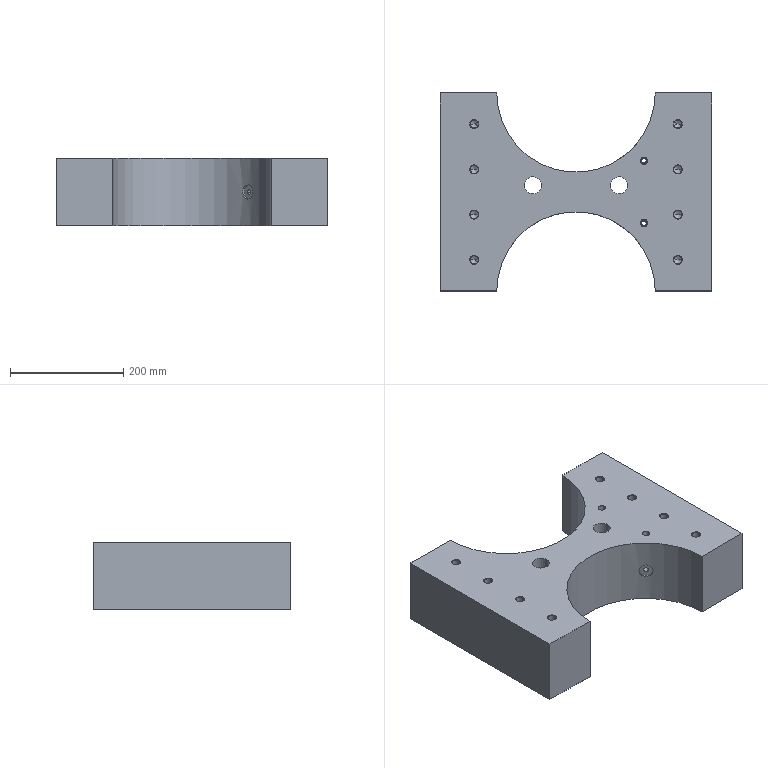Part | SolidWorks | features ICE 4, HoleWzd 3, Extrusion 1, MirrorPattern 1 | 1 solid | 112 faces | box 480 x 350 x 120 mm | volume 12537769 mm3 | cone 56 | cylinder 42 | plane 14 | commonest cylinder face diameters 14 x16 8 x8 10.7 x8 25 x4 30 x4 280 x2